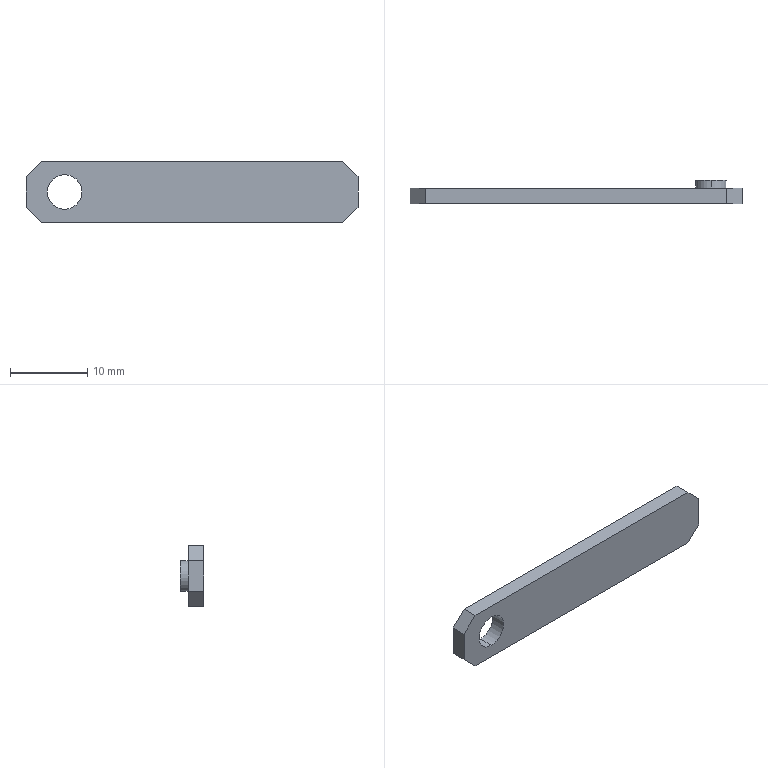Part | SolidWorks | features Chamfer 2, ICE 2, Extrusion 1 | 1 solid | 15 faces | box 43 x 3 x 8 mm | volume 652.758 mm3 | plane 11 | cylinder 4 | commonest cylinder face diameters 4 x2 4.5 x2
STEP:
#1=CARTESIAN_POINT('',(29.307,3.,-1.484));
#2=VERTEX_POINT('',#1);
#3=CARTESIAN_POINT('',(29.307,3.,-5.484));
#4=VERTEX_POINT('',#3);
#5=CARTESIAN_POINT('',(29.307,3.,-3.484));
#6=DIRECTION('',(0.,1.,0.));
#7=DIRECTION('',(0.,0.,1.));
#8=AXIS2_PLACEMENT_3D('',#5,#6,#7);
#9=CIRCLE('',#8,2.);
#10=EDGE_CURVE('',#2,#4,#9,.T.);
#11=ORIENTED_EDGE('',*,*,#10,.F.);
#12=CARTESIAN_POINT('',(29.307,2.,-1.484));
#13=VERTEX_POINT('',#12);
#14=CARTESIAN_POINT('',(29.307,3.,-1.484));
#15=DIRECTION('',(0.,-1.,0.));
#16=VECTOR('',#15,1000.);
#17=LINE('',#14,#16);
#18=EDGE_CURVE('',#2,#13,#17,.T.);
#19=ORIENTED_EDGE('',*,*,#18,.T.);
#20=CARTESIAN_POINT('',(29.307,2.,-5.484));
#21=VERTEX_POINT('',#20);
#22=CARTESIAN_POINT('',(29.307,2.,-3.484));
#23=DIRECTION('',(0.,1.,0.));
#24=DIRECTION('',(0.,0.,1.));
#25=AXIS2_PLACEMENT_3D('',#22,#23,#24);
#26=CIRCLE('',#25,2.);
#27=EDGE_CURVE('',#13,#21,#26,.T.);
#28=ORIENTED_EDGE('',*,*,#27,.T.);
#29=CARTESIAN_POINT('',(29.307,3.,-5.484));
#30=DIRECTION('',(0.,-1.,0.));
#31=VECTOR('',#30,1000.);
#32=LINE('',#29,#31);
#33=EDGE_CURVE('',#4,#21,#32,.T.);
#34=ORIENTED_EDGE('',*,*,#33,.F.);
#35=EDGE_LOOP('',(#11,#19,#28,#34));
#36=FACE_OUTER_BOUND('',#35,.T.);
#37=CARTESIAN_POINT('',(29.307,3.,-3.484));
#38=DIRECTION('',(0.,-1.,0.));
#39=DIRECTION('',(0.,0.,-1.));
#40=AXIS2_PLACEMENT_3D('',#37,#38,#39);
#41=CYLINDRICAL_SURFACE('',#40,2.);
#42=ADVANCED_FACE('',(#36),#41,.T.);
#43=CARTESIAN_POINT('',(-4.693,0.,-5.734));
#44=VERTEX_POINT('',#43);
#45=CARTESIAN_POINT('',(-4.693,0.,-1.234));
#46=VERTEX_POINT('',#45);
#47=CARTESIAN_POINT('',(-4.693,0.,-3.484));
#48=DIRECTION('',(0.,1.,0.));
#49=DIRECTION('',(0.,0.,1.));
#50=AXIS2_PLACEMENT_3D('',#47,#48,#49);
#51=CIRCLE('',#50,2.25);
#52=EDGE_CURVE('',#44,#46,#51,.T.);
#53=ORIENTED_EDGE('',*,*,#52,.F.);
#54=CARTESIAN_POINT('',(-4.693,2.,-5.734));
#55=VERTEX_POINT('',#54);
#56=CARTESIAN_POINT('',(-4.693,0.,-5.734));
#57=DIRECTION('',(0.,1.,0.));
#58=VECTOR('',#57,1000.);
#59=LINE('',#56,#58);
#60=EDGE_CURVE('',#44,#55,#59,.T.);
#61=ORIENTED_EDGE('',*,*,#60,.T.);
#62=CARTESIAN_POINT('',(-4.693,2.,-1.234));
#63=VERTEX_POINT('',#62);
#64=CARTESIAN_POINT('',(-4.693,2.,-3.484));
#65=DIRECTION('',(0.,1.,0.));
#66=DIRECTION('',(0.,0.,1.));
#67=AXIS2_PLACEMENT_3D('',#64,#65,#66);
#68=CIRCLE('',#67,2.25);
#69=EDGE_CURVE('',#55,#63,#68,.T.);
#70=ORIENTED_EDGE('',*,*,#69,.T.);
#71=CARTESIAN_POINT('',(-4.693,0.,-1.234));
#72=DIRECTION('',(0.,1.,0.));
#73=VECTOR('',#72,1000.);
#74=LINE('',#71,#73);
#75=EDGE_CURVE('',#46,#63,#74,.T.);
#76=ORIENTED_EDGE('',*,*,#75,.F.);
#77=EDGE_LOOP('',(#53,#61,#70,#76));
#78=FACE_OUTER_BOUND('',#77,.T.);
#79=CARTESIAN_POINT('',(-4.693,0.,-3.484));
#80=DIRECTION('',(0.,1.,0.));
#81=DIRECTION('',(0.,0.,1.));
#82=AXIS2_PLACEMENT_3D('',#79,#80,#81);
#83=CYLINDRICAL_SURFACE('',#82,2.25);
#84=ADVANCED_FACE('',(#78),#83,.F.);
#85=CARTESIAN_POINT('',(33.307,2.,-1.484));
#86=VERTEX_POINT('',#85);
#87=CARTESIAN_POINT('',(33.307,2.,-5.484));
#88=VERTEX_POINT('',#87);
#89=CARTESIAN_POINT('',(33.307,2.,-7.484));
#90=DIRECTION('',(0.,0.,-1.));
#91=VECTOR('',#90,1000.);
#92=LINE('',#89,#91);
#93=EDGE_CURVE('',#86,#88,#92,.T.);
#94=ORIENTED_EDGE('',*,*,#93,.T.);
#95=CARTESIAN_POINT('',(31.307,2.,-7.484));
#96=VERTEX_POINT('',#95);
#97=CARTESIAN_POINT('',(19.396,2.,-19.396));
#98=DIRECTION('',(-0.7071,0.,-0.7071));
#99=VECTOR('',#98,1000.);
#100=LINE('',#97,#99);
#101=EDGE_CURVE('',#88,#96,#100,.T.);
#102=ORIENTED_EDGE('',*,*,#101,.T.);
#103=CARTESIAN_POINT('',(-7.693,2.,-7.484));
#104=VERTEX_POINT('',#103);
#105=CARTESIAN_POINT('',(-9.693,2.,-7.484));
#106=DIRECTION('',(-1.,0.,0.));
#107=VECTOR('',#106,1000.);
#108=LINE('',#105,#107);
#109=EDGE_CURVE('',#96,#104,#108,.T.);
#110=ORIENTED_EDGE('',*,*,#109,.T.);
#111=CARTESIAN_POINT('',(-9.693,2.,-5.484));
#112=VERTEX_POINT('',#111);
#113=CARTESIAN_POINT('',(-7.589,2.,-7.589));
#114=DIRECTION('',(-0.7071,0.,0.7071));
#115=VECTOR('',#114,1000.);
#116=LINE('',#113,#115);
#117=EDGE_CURVE('',#104,#112,#116,.T.);
#118=ORIENTED_EDGE('',*,*,#117,.T.);
#119=CARTESIAN_POINT('',(-9.693,2.,-1.484));
#120=VERTEX_POINT('',#119);
#121=CARTESIAN_POINT('',(-9.693,2.,-7.484));
#122=DIRECTION('',(0.,0.,1.));
#123=VECTOR('',#122,1000.);
#124=LINE('',#121,#123);
#125=EDGE_CURVE('',#112,#120,#124,.T.);
#126=ORIENTED_EDGE('',*,*,#125,.T.);
#127=CARTESIAN_POINT('',(-7.693,2.,0.5156));
#128=VERTEX_POINT('',#127);
#129=CARTESIAN_POINT('',(-4.104,2.,4.104));
#130=DIRECTION('',(0.7071,0.,0.7071));
#131=VECTOR('',#130,1000.);
#132=LINE('',#129,#131);
#133=EDGE_CURVE('',#120,#128,#132,.T.);
#134=ORIENTED_EDGE('',*,*,#133,.T.);
#135=CARTESIAN_POINT('',(31.307,2.,0.5156));
#136=VERTEX_POINT('',#135);
#137=CARTESIAN_POINT('',(-9.693,2.,0.5156));
#138=DIRECTION('',(1.,0.,0.));
#139=VECTOR('',#138,1000.);
#140=LINE('',#137,#139);
#141=EDGE_CURVE('',#128,#136,#140,.T.);
#142=ORIENTED_EDGE('',*,*,#141,.T.);
#143=CARTESIAN_POINT('',(15.911,2.,15.911));
#144=DIRECTION('',(0.7071,0.,-0.7071));
#145=VECTOR('',#144,1000.);
#146=LINE('',#143,#145);
#147=EDGE_CURVE('',#136,#86,#146,.T.);
#148=ORIENTED_EDGE('',*,*,#147,.T.);
#149=EDGE_LOOP('',(#94,#102,#110,#118,#126,#134,#142,#148));
#150=FACE_OUTER_BOUND('',#149,.T.);
#151=CARTESIAN_POINT('',(-4.693,2.,-3.484));
#152=DIRECTION('',(0.,1.,0.));
#153=DIRECTION('',(0.,0.,1.));
#154=AXIS2_PLACEMENT_3D('',#151,#152,#153);
#155=CIRCLE('',#154,2.25);
#156=EDGE_CURVE('',#63,#55,#155,.T.);
#157=ORIENTED_EDGE('',*,*,#156,.F.);
#158=ORIENTED_EDGE('',*,*,#69,.F.);
#159=EDGE_LOOP('',(#157,#158));
#160=FACE_BOUND('',#159,.T.);
#161=CARTESIAN_POINT('',(29.307,2.,-3.484));
#162=DIRECTION('',(0.,1.,0.));
#163=DIRECTION('',(0.,0.,1.));
#164=AXIS2_PLACEMENT_3D('',#161,#162,#163);
#165=CIRCLE('',#164,2.);
#166=EDGE_CURVE('',#21,#13,#165,.T.);
#167=ORIENTED_EDGE('',*,*,#166,.F.);
#168=ORIENTED_EDGE('',*,*,#27,.F.);
#169=EDGE_LOOP('',(#167,#168));
#170=FACE_BOUND('',#169,.T.);
#171=CARTESIAN_POINT('',(0.,2.,0.));
#172=DIRECTION('',(0.,1.,0.));
#173=DIRECTION('',(0.,0.,1.));
#174=AXIS2_PLACEMENT_3D('',#171,#172,#173);
#175=PLANE('',#174);
#176=ADVANCED_FACE('',(#150,#160,#170),#175,.T.);
#177=ORIENTED_EDGE('',*,*,#125,.F.);
#178=CARTESIAN_POINT('',(-9.693,0.,-5.484));
#179=VERTEX_POINT('',#178);
#180=CARTESIAN_POINT('',(-9.693,2.,-5.484));
#181=DIRECTION('',(0.,-1.,0.));
#182=VECTOR('',#181,1000.);
#183=LINE('',#180,#182);
#184=EDGE_CURVE('',#112,#179,#183,.T.);
#185=ORIENTED_EDGE('',*,*,#184,.T.);
#186=CARTESIAN_POINT('',(-9.693,0.,-1.484));
#187=VERTEX_POINT('',#186);
#188=CARTESIAN_POINT('',(-9.693,0.,-7.484));
#189=DIRECTION('',(0.,0.,1.));
#190=VECTOR('',#189,1000.);
#191=LINE('',#188,#190);
#192=EDGE_CURVE('',#179,#187,#191,.T.);
#193=ORIENTED_EDGE('',*,*,#192,.T.);
#194=CARTESIAN_POINT('',(-9.693,2.,-1.484));
#195=DIRECTION('',(0.,1.,0.));
#196=VECTOR('',#195,1000.);
#197=LINE('',#194,#196);
#198=EDGE_CURVE('',#187,#120,#197,.T.);
#199=ORIENTED_EDGE('',*,*,#198,.T.);
#200=EDGE_LOOP('',(#177,#185,#193,#199));
#201=FACE_OUTER_BOUND('',#200,.T.);
#202=CARTESIAN_POINT('',(-9.693,2.,-7.484));
#203=DIRECTION('',(1.,0.,0.));
#204=DIRECTION('',(0.,0.,-1.));
#205=AXIS2_PLACEMENT_3D('',#202,#203,#204);
#206=PLANE('',#205);
#207=ADVANCED_FACE('',(#201),#206,.F.);
#208=CARTESIAN_POINT('',(-7.693,0.,0.5156));
#209=VERTEX_POINT('',#208);
#210=CARTESIAN_POINT('',(31.307,0.,0.5156));
#211=VERTEX_POINT('',#210);
#212=CARTESIAN_POINT('',(-9.693,0.,0.5156));
#213=DIRECTION('',(1.,0.,0.));
#214=VECTOR('',#213,1000.);
#215=LINE('',#212,#214);
#216=EDGE_CURVE('',#209,#211,#215,.T.);
#217=ORIENTED_EDGE('',*,*,#216,.T.);
#218=CARTESIAN_POINT('',(31.307,2.,0.5156));
#219=DIRECTION('',(0.,1.,0.));
#220=VECTOR('',#219,1000.);
#221=LINE('',#218,#220);
#222=EDGE_CURVE('',#211,#136,#221,.T.);
#223=ORIENTED_EDGE('',*,*,#222,.T.);
#224=ORIENTED_EDGE('',*,*,#141,.F.);
#225=CARTESIAN_POINT('',(-7.693,2.,0.5156));
#226=DIRECTION('',(0.,-1.,0.));
#227=VECTOR('',#226,1000.);
#228=LINE('',#225,#227);
#229=EDGE_CURVE('',#128,#209,#228,.T.);
#230=ORIENTED_EDGE('',*,*,#229,.T.);
#231=EDGE_LOOP('',(#217,#223,#224,#230));
#232=FACE_OUTER_BOUND('',#231,.T.);
#233=CARTESIAN_POINT('',(-9.693,2.,0.5156));
#234=DIRECTION('',(0.,0.,-1.));
#235=DIRECTION('',(-1.,0.,0.));
#236=AXIS2_PLACEMENT_3D('',#233,#234,#235);
#237=PLANE('',#236);
#238=ADVANCED_FACE('',(#232),#237,.F.);
#239=CARTESIAN_POINT('',(33.307,0.,-1.484));
#240=VERTEX_POINT('',#239);
#241=CARTESIAN_POINT('',(33.307,0.,-5.484));
#242=VERTEX_POINT('',#241);
#243=CARTESIAN_POINT('',(33.307,0.,-7.484));
#244=DIRECTION('',(0.,0.,-1.));
#245=VECTOR('',#244,1000.);
#246=LINE('',#243,#245);
#247=EDGE_CURVE('',#240,#242,#246,.T.);
#248=ORIENTED_EDGE('',*,*,#247,.T.);
#249=CARTESIAN_POINT('',(33.307,2.,-5.484));
#250=DIRECTION('',(0.,1.,0.));
#251=VECTOR('',#250,1000.);
#252=LINE('',#249,#251);
#253=EDGE_CURVE('',#242,#88,#252,.T.);
#254=ORIENTED_EDGE('',*,*,#253,.T.);
#255=ORIENTED_EDGE('',*,*,#93,.F.);
#256=CARTESIAN_POINT('',(33.307,2.,-1.484));
#257=DIRECTION('',(0.,-1.,0.));
#258=VECTOR('',#257,1000.);
#259=LINE('',#256,#258);
#260=EDGE_CURVE('',#86,#240,#259,.T.);
#261=ORIENTED_EDGE('',*,*,#260,.T.);
#262=EDGE_LOOP('',(#248,#254,#255,#261));
#263=FACE_OUTER_BOUND('',#262,.T.);
#264=CARTESIAN_POINT('',(33.307,2.,-7.484));
#265=DIRECTION('',(-1.,0.,0.));
#266=DIRECTION('',(0.,0.,1.));
#267=AXIS2_PLACEMENT_3D('',#264,#265,#266);
#268=PLANE('',#267);
#269=ADVANCED_FACE('',(#263),#268,.F.);
#270=ORIENTED_EDGE('',*,*,#109,.F.);
#271=CARTESIAN_POINT('',(31.307,0.,-7.484));
#272=VERTEX_POINT('',#271);
#273=CARTESIAN_POINT('',(31.307,2.,-7.484));
#274=DIRECTION('',(0.,-1.,0.));
#275=VECTOR('',#274,1000.);
#276=LINE('',#273,#275);
#277=EDGE_CURVE('',#96,#272,#276,.T.);
#278=ORIENTED_EDGE('',*,*,#277,.T.);
#279=CARTESIAN_POINT('',(-7.693,0.,-7.484));
#280=VERTEX_POINT('',#279);
#281=CARTESIAN_POINT('',(-9.693,0.,-7.484));
#282=DIRECTION('',(-1.,0.,0.));
#283=VECTOR('',#282,1000.);
#284=LINE('',#281,#283);
#285=EDGE_CURVE('',#272,#280,#284,.T.);
#286=ORIENTED_EDGE('',*,*,#285,.T.);
#287=CARTESIAN_POINT('',(-7.693,2.,-7.484));
#288=DIRECTION('',(0.,1.,0.));
#289=VECTOR('',#288,1000.);
#290=LINE('',#287,#289);
#291=EDGE_CURVE('',#280,#104,#290,.T.);
#292=ORIENTED_EDGE('',*,*,#291,.T.);
#293=EDGE_LOOP('',(#270,#278,#286,#292));
#294=FACE_OUTER_BOUND('',#293,.T.);
#295=CARTESIAN_POINT('',(-9.693,2.,-7.484));
#296=DIRECTION('',(0.,0.,1.));
#297=DIRECTION('',(1.,0.,0.));
#298=AXIS2_PLACEMENT_3D('',#295,#296,#297);
#299=PLANE('',#298);
#300=ADVANCED_FACE('',(#294),#299,.F.);
#301=CARTESIAN_POINT('',(-4.693,0.,-3.484));
#302=DIRECTION('',(0.,1.,0.));
#303=DIRECTION('',(0.,0.,1.));
#304=AXIS2_PLACEMENT_3D('',#301,#302,#303);
#305=CIRCLE('',#304,2.25);
#306=EDGE_CURVE('',#46,#44,#305,.T.);
#307=ORIENTED_EDGE('',*,*,#306,.T.);
#308=ORIENTED_EDGE('',*,*,#52,.T.);
#309=EDGE_LOOP('',(#307,#308));
#310=FACE_BOUND('',#309,.T.);
#311=ORIENTED_EDGE('',*,*,#285,.F.);
#312=CARTESIAN_POINT('',(31.307,0.,-7.484));
#313=DIRECTION('',(0.7071,0.,0.7071));
#314=VECTOR('',#313,1000.);
#315=LINE('',#312,#314);
#316=EDGE_CURVE('',#272,#242,#315,.T.);
#317=ORIENTED_EDGE('',*,*,#316,.T.);
#318=ORIENTED_EDGE('',*,*,#247,.F.);
#319=CARTESIAN_POINT('',(33.307,0.,-1.484));
#320=DIRECTION('',(-0.7071,0.,0.7071));
#321=VECTOR('',#320,1000.);
#322=LINE('',#319,#321);
#323=EDGE_CURVE('',#240,#211,#322,.T.);
#324=ORIENTED_EDGE('',*,*,#323,.T.);
#325=ORIENTED_EDGE('',*,*,#216,.F.);
#326=CARTESIAN_POINT('',(-7.693,0.,0.5156));
#327=DIRECTION('',(-0.7071,0.,-0.7071));
#328=VECTOR('',#327,1000.);
#329=LINE('',#326,#328);
#330=EDGE_CURVE('',#209,#187,#329,.T.);
#331=ORIENTED_EDGE('',*,*,#330,.T.);
#332=ORIENTED_EDGE('',*,*,#192,.F.);
#333=CARTESIAN_POINT('',(-9.693,0.,-5.484));
#334=DIRECTION('',(0.7071,0.,-0.7071));
#335=VECTOR('',#334,1000.);
#336=LINE('',#333,#335);
#337=EDGE_CURVE('',#179,#280,#336,.T.);
#338=ORIENTED_EDGE('',*,*,#337,.T.);
#339=EDGE_LOOP('',(#311,#317,#318,#324,#325,#331,#332,#338));
#340=FACE_OUTER_BOUND('',#339,.T.);
#341=CARTESIAN_POINT('',(0.,0.,0.));
#342=DIRECTION('',(0.,1.,0.));
#343=DIRECTION('',(0.,0.,1.));
#344=AXIS2_PLACEMENT_3D('',#341,#342,#343);
#345=PLANE('',#344);
#346=ADVANCED_FACE('',(#310,#340),#345,.F.);
#347=ORIENTED_EDGE('',*,*,#60,.F.);
#348=ORIENTED_EDGE('',*,*,#306,.F.);
#349=ORIENTED_EDGE('',*,*,#75,.T.);
#350=ORIENTED_EDGE('',*,*,#156,.T.);
#351=EDGE_LOOP('',(#347,#348,#349,#350));
#352=FACE_OUTER_BOUND('',#351,.T.);
#353=CARTESIAN_POINT('',(-4.693,0.,-3.484));
#354=DIRECTION('',(0.,1.,0.));
#355=DIRECTION('',(0.,0.,1.));
#356=AXIS2_PLACEMENT_3D('',#353,#354,#355);
#357=CYLINDRICAL_SURFACE('',#356,2.25);
#358=ADVANCED_FACE('',(#352),#357,.F.);
#359=ORIENTED_EDGE('',*,*,#18,.F.);
#360=CARTESIAN_POINT('',(29.307,3.,-3.484));
#361=DIRECTION('',(0.,1.,0.));
#362=DIRECTION('',(0.,0.,1.));
#363=AXIS2_PLACEMENT_3D('',#360,#361,#362);
#364=CIRCLE('',#363,2.);
#365=EDGE_CURVE('',#4,#2,#364,.T.);
#366=ORIENTED_EDGE('',*,*,#365,.F.);
#367=ORIENTED_EDGE('',*,*,#33,.T.);
#368=ORIENTED_EDGE('',*,*,#166,.T.);
#369=EDGE_LOOP('',(#359,#366,#367,#368));
#370=FACE_OUTER_BOUND('',#369,.T.);
#371=CARTESIAN_POINT('',(29.307,3.,-3.484));
#372=DIRECTION('',(0.,-1.,0.));
#373=DIRECTION('',(0.,0.,-1.));
#374=AXIS2_PLACEMENT_3D('',#371,#372,#373);
#375=CYLINDRICAL_SURFACE('',#374,2.);
#376=ADVANCED_FACE('',(#370),#375,.T.);
#377=ORIENTED_EDGE('',*,*,#365,.T.);
#378=ORIENTED_EDGE('',*,*,#10,.T.);
#379=EDGE_LOOP('',(#377,#378));
#380=FACE_OUTER_BOUND('',#379,.T.);
#381=CARTESIAN_POINT('',(29.307,3.,-3.484));
#382=DIRECTION('',(0.,1.,0.));
#383=DIRECTION('',(0.,0.,1.));
#384=AXIS2_PLACEMENT_3D('',#381,#382,#383);
#385=PLANE('',#384);
#386=ADVANCED_FACE('',(#380),#385,.T.);
#387=ORIENTED_EDGE('',*,*,#101,.F.);
#388=ORIENTED_EDGE('',*,*,#253,.F.);
#389=ORIENTED_EDGE('',*,*,#316,.F.);
#390=ORIENTED_EDGE('',*,*,#277,.F.);
#391=EDGE_LOOP('',(#387,#388,#389,#390));
#392=FACE_OUTER_BOUND('',#391,.T.);
#393=CARTESIAN_POINT('',(31.307,2.,-7.484));
#394=DIRECTION('',(-0.7071,0.,0.7071));
#395=DIRECTION('',(0.,-1.,0.));
#396=AXIS2_PLACEMENT_3D('',#393,#394,#395);
#397=PLANE('',#396);
#398=ADVANCED_FACE('',(#392),#397,.F.);
#399=ORIENTED_EDGE('',*,*,#147,.F.);
#400=ORIENTED_EDGE('',*,*,#222,.F.);
#401=ORIENTED_EDGE('',*,*,#323,.F.);
#402=ORIENTED_EDGE('',*,*,#260,.F.);
#403=EDGE_LOOP('',(#399,#400,#401,#402));
#404=FACE_OUTER_BOUND('',#403,.T.);
#405=CARTESIAN_POINT('',(33.307,2.,-1.484));
#406=DIRECTION('',(-0.7071,0.,-0.7071));
#407=DIRECTION('',(0.,-1.,0.));
#408=AXIS2_PLACEMENT_3D('',#405,#406,#407);
#409=PLANE('',#408);
#410=ADVANCED_FACE('',(#404),#409,.F.);
#411=ORIENTED_EDGE('',*,*,#117,.F.);
#412=ORIENTED_EDGE('',*,*,#291,.F.);
#413=ORIENTED_EDGE('',*,*,#337,.F.);
#414=ORIENTED_EDGE('',*,*,#184,.F.);
#415=EDGE_LOOP('',(#411,#412,#413,#414));
#416=FACE_OUTER_BOUND('',#415,.T.);
#417=CARTESIAN_POINT('',(-9.693,2.,-5.484));
#418=DIRECTION('',(0.7071,0.,0.7071));
#419=DIRECTION('',(0.,-1.,0.));
#420=AXIS2_PLACEMENT_3D('',#417,#418,#419);
#421=PLANE('',#420);
#422=ADVANCED_FACE('',(#416),#421,.F.);
#423=ORIENTED_EDGE('',*,*,#133,.F.);
#424=ORIENTED_EDGE('',*,*,#198,.F.);
#425=ORIENTED_EDGE('',*,*,#330,.F.);
#426=ORIENTED_EDGE('',*,*,#229,.F.);
#427=EDGE_LOOP('',(#423,#424,#425,#426));
#428=FACE_OUTER_BOUND('',#427,.T.);
#429=CARTESIAN_POINT('',(-7.693,2.,0.5156));
#430=DIRECTION('',(0.7071,0.,-0.7071));
#431=DIRECTION('',(0.,-1.,0.));
#432=AXIS2_PLACEMENT_3D('',#429,#430,#431);
#433=PLANE('',#432);
#434=ADVANCED_FACE('',(#428),#433,.F.);
#435=CLOSED_SHELL('',(#42,#84,#176,#207,#238,#269,#300,#346,#358,#376,#386,#398,#410,#422,#434));
#436=MANIFOLD_SOLID_BREP('',#435);
#437=CARTESIAN_POINT('',(0.,0.,0.));
#438=DIRECTION('',(0.,0.,1.));
#439=DIRECTION('',(1.,0.,0.));
#440=AXIS2_PLACEMENT_3D('',#437,#438,#439);
#441=(LENGTH_UNIT()NAMED_UNIT(*)SI_UNIT(.MILLI.,.METRE.));
#442=UNCERTAINTY_MEASURE_WITH_UNIT(LENGTH_MEASURE(0.00001),#441,'','');
#443=(NAMED_UNIT(*)PLANE_ANGLE_UNIT()SI_UNIT($,.RADIAN.));
#444=(NAMED_UNIT(*)SI_UNIT($,.STERADIAN.)SOLID_ANGLE_UNIT());
#445=(GEOMETRIC_REPRESENTATION_CONTEXT(3)GLOBAL_UNCERTAINTY_ASSIGNED_CONTEXT((#442))GLOBAL_UNIT_ASSIGNED_CONTEXT((#441,#443,#444))REPRESENTATION_CONTEXT('',''));
#446=ADVANCED_BREP_SHAPE_REPRESENTATION('',(#436,#440),#445);